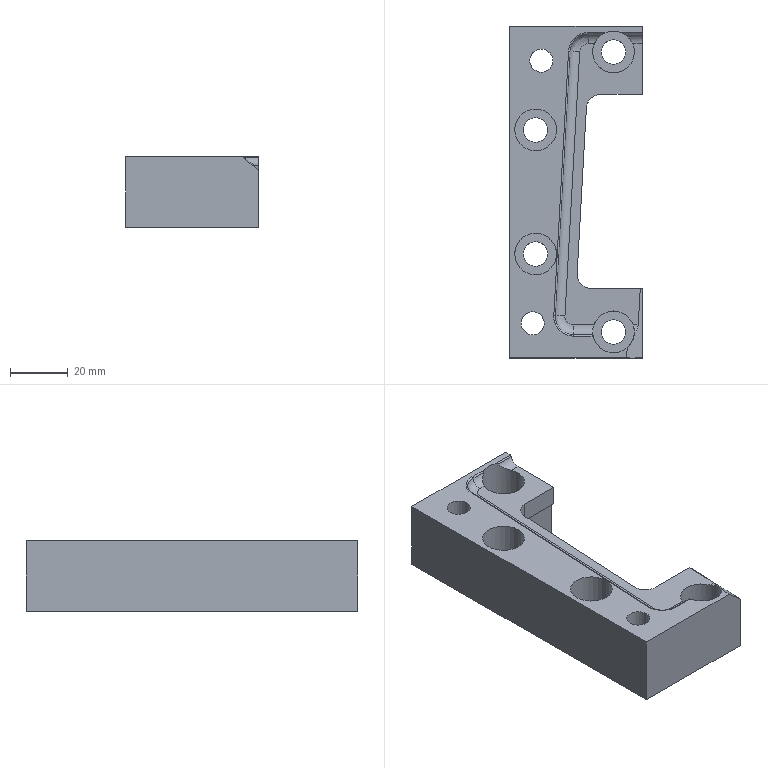Part | NX | features solid 2 | 1 solid | 47 faces | box 46 x 115 x 24.5 mm | volume 75908 mm3 | plane 20 | cylinder 19 | torus 4 | spline 4 | commonest cylinder face diameters 7 x5 1 x4 8.5 x4 14.5 x4 8.001 x2